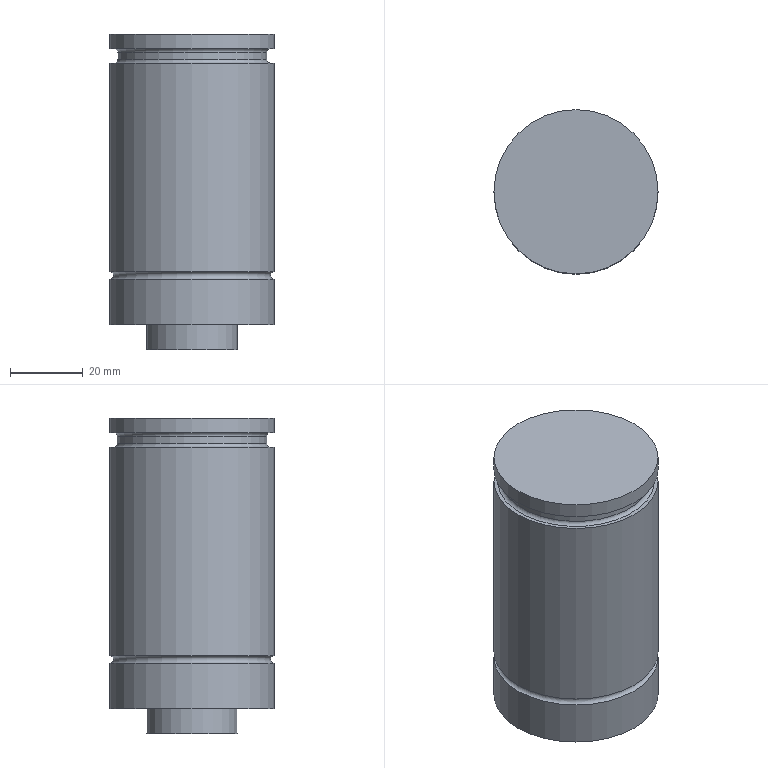Part | NX | features solid 2 | 1 solid | 13 faces | box 45.2 x 45.2 x 87 mm | volume 130556 mm3 | cylinder 5 | plane 5 | torus 3 | commonest cylinder face diameters 45.2 x3 25 x1 41.2 x1
STEP:
#1=CARTESIAN_POINT('',(-1182.6,-595.,9.));
#2=VERTEX_POINT('',#1);
#3=CARTESIAN_POINT('',(-1160.,-595.,9.));
#4=DIRECTION('',(0.,0.,-1.));
#5=DIRECTION('',(-1.,0.,0.));
#6=AXIS2_PLACEMENT_3D('',#3,#4,#5);
#7=CIRCLE('',#6,22.6);
#8=EDGE_CURVE('',#2,#2,#7,.T.);
#9=ORIENTED_EDGE('',*,*,#8,.T.);
#10=EDGE_LOOP('',(#9));
#11=FACE_BOUND('',#10,.T.);
#12=CARTESIAN_POINT('',(-1137.4,-595.,-48.5));
#13=VERTEX_POINT('',#12);
#14=CARTESIAN_POINT('',(-1160.,-595.,-48.5));
#15=DIRECTION('',(0.,0.,1.));
#16=DIRECTION('',(1.,0.,0.));
#17=AXIS2_PLACEMENT_3D('',#14,#15,#16);
#18=CIRCLE('',#17,22.6);
#19=EDGE_CURVE('',#13,#13,#18,.T.);
#20=ORIENTED_EDGE('',*,*,#19,.T.);
#21=EDGE_LOOP('',(#20));
#22=FACE_BOUND('',#21,.T.);
#23=CARTESIAN_POINT('',(-1160.,-595.,-63.));
#24=DIRECTION('',(0.,0.,1.));
#25=DIRECTION('',(1.,0.,0.));
#26=AXIS2_PLACEMENT_3D('',#23,#24,#25);
#27=CYLINDRICAL_SURFACE('',#26,22.6);
#28=ADVANCED_FACE('',(#11,#22),#27,.T.);
#29=CARTESIAN_POINT('',(-1172.5,-595.,-63.));
#30=VERTEX_POINT('',#29);
#31=CARTESIAN_POINT('',(-1160.,-595.,-63.));
#32=DIRECTION('',(0.,0.,-1.));
#33=DIRECTION('',(-1.,0.,0.));
#34=AXIS2_PLACEMENT_3D('',#31,#32,#33);
#35=CIRCLE('',#34,12.5);
#36=EDGE_CURVE('',#30,#30,#35,.T.);
#37=ORIENTED_EDGE('',*,*,#36,.F.);
#38=EDGE_LOOP('',(#37));
#39=FACE_BOUND('',#38,.T.);
#40=CARTESIAN_POINT('',(-1137.4,-595.,-63.));
#41=VERTEX_POINT('',#40);
#42=CARTESIAN_POINT('',(-1160.,-595.,-63.));
#43=DIRECTION('',(0.,0.,1.));
#44=DIRECTION('',(1.,0.,0.));
#45=AXIS2_PLACEMENT_3D('',#42,#43,#44);
#46=CIRCLE('',#45,22.6);
#47=EDGE_CURVE('',#41,#41,#46,.T.);
#48=ORIENTED_EDGE('',*,*,#47,.F.);
#49=EDGE_LOOP('',(#48));
#50=FACE_BOUND('',#49,.T.);
#51=CARTESIAN_POINT('',(-1160.,-595.,-63.));
#52=DIRECTION('',(0.,0.,-1.));
#53=DIRECTION('',(-1.,0.,0.));
#54=AXIS2_PLACEMENT_3D('',#51,#52,#53);
#55=PLANE('',#54);
#56=ADVANCED_FACE('',(#39,#50),#55,.T.);
#57=CARTESIAN_POINT('',(-1137.4,-595.,-50.5));
#58=VERTEX_POINT('',#57);
#59=CARTESIAN_POINT('',(-1160.,-595.,-50.5));
#60=DIRECTION('',(0.,0.,1.));
#61=DIRECTION('',(1.,0.,0.));
#62=AXIS2_PLACEMENT_3D('',#59,#60,#61);
#63=CIRCLE('',#62,22.6);
#64=EDGE_CURVE('',#58,#58,#63,.T.);
#65=ORIENTED_EDGE('',*,*,#64,.F.);
#66=EDGE_LOOP('',(#65));
#67=FACE_BOUND('',#66,.T.);
#68=ORIENTED_EDGE('',*,*,#47,.T.);
#69=EDGE_LOOP('',(#68));
#70=FACE_BOUND('',#69,.T.);
#71=CARTESIAN_POINT('',(-1160.,-595.,-63.));
#72=DIRECTION('',(0.,0.,1.));
#73=DIRECTION('',(1.,0.,0.));
#74=AXIS2_PLACEMENT_3D('',#71,#72,#73);
#75=CYLINDRICAL_SURFACE('',#74,22.6);
#76=ADVANCED_FACE('',(#67,#70),#75,.T.);
#77=CARTESIAN_POINT('',(-1147.5,-595.,-70.));
#78=VERTEX_POINT('',#77);
#79=CARTESIAN_POINT('',(-1160.,-595.,-70.));
#80=DIRECTION('',(0.,0.,1.));
#81=DIRECTION('',(1.,0.,0.));
#82=AXIS2_PLACEMENT_3D('',#79,#80,#81);
#83=CIRCLE('',#82,12.5);
#84=EDGE_CURVE('',#78,#78,#83,.T.);
#85=ORIENTED_EDGE('',*,*,#84,.F.);
#86=EDGE_LOOP('',(#85));
#87=FACE_BOUND('',#86,.T.);
#88=CARTESIAN_POINT('',(-1160.,-595.,-70.));
#89=DIRECTION('',(0.,0.,-1.));
#90=DIRECTION('',(-1.,0.,0.));
#91=AXIS2_PLACEMENT_3D('',#88,#89,#90);
#92=PLANE('',#91);
#93=ADVANCED_FACE('',(#87),#92,.T.);
#94=ORIENTED_EDGE('',*,*,#36,.T.);
#95=EDGE_LOOP('',(#94));
#96=FACE_BOUND('',#95,.T.);
#97=ORIENTED_EDGE('',*,*,#84,.T.);
#98=EDGE_LOOP('',(#97));
#99=FACE_BOUND('',#98,.T.);
#100=CARTESIAN_POINT('',(-1160.,-595.,-70.));
#101=DIRECTION('',(0.,0.,1.));
#102=DIRECTION('',(1.,0.,0.));
#103=AXIS2_PLACEMENT_3D('',#100,#101,#102);
#104=CYLINDRICAL_SURFACE('',#103,12.5);
#105=ADVANCED_FACE('',(#96,#99),#104,.T.);
#106=ORIENTED_EDGE('',*,*,#19,.F.);
#107=EDGE_LOOP('',(#106));
#108=FACE_BOUND('',#107,.T.);
#109=ORIENTED_EDGE('',*,*,#64,.T.);
#110=EDGE_LOOP('',(#109));
#111=FACE_BOUND('',#110,.T.);
#112=CARTESIAN_POINT('',(-1160.,-595.,-49.5));
#113=DIRECTION('',(0.,0.,-1.));
#114=DIRECTION('',(-1.,0.,0.));
#115=AXIS2_PLACEMENT_3D('',#112,#113,#114);
#116=TOROIDAL_SURFACE('',#115,22.6,1.);
#117=ADVANCED_FACE('',(#108,#111),#116,.F.);
#118=CARTESIAN_POINT('',(-1139.4,-595.,10.));
#119=VERTEX_POINT('',#118);
#120=CARTESIAN_POINT('',(-1160.,-595.,10.));
#121=DIRECTION('',(0.,0.,1.));
#122=DIRECTION('',(1.,0.,0.));
#123=AXIS2_PLACEMENT_3D('',#120,#121,#122);
#124=CIRCLE('',#123,20.6);
#125=EDGE_CURVE('',#119,#119,#124,.T.);
#126=ORIENTED_EDGE('',*,*,#125,.T.);
#127=EDGE_LOOP('',(#126));
#128=FACE_BOUND('',#127,.T.);
#129=CARTESIAN_POINT('',(-1139.4,-595.,12.));
#130=VERTEX_POINT('',#129);
#131=CARTESIAN_POINT('',(-1160.,-595.,12.));
#132=DIRECTION('',(0.,0.,1.));
#133=DIRECTION('',(1.,0.,0.));
#134=AXIS2_PLACEMENT_3D('',#131,#132,#133);
#135=CIRCLE('',#134,20.6);
#136=EDGE_CURVE('',#130,#130,#135,.F.);
#137=ORIENTED_EDGE('',*,*,#136,.T.);
#138=EDGE_LOOP('',(#137));
#139=FACE_BOUND('',#138,.T.);
#140=CARTESIAN_POINT('',(-1160.,-595.,13.));
#141=DIRECTION('',(0.,0.,-1.));
#142=DIRECTION('',(-1.,0.,0.));
#143=AXIS2_PLACEMENT_3D('',#140,#141,#142);
#144=CYLINDRICAL_SURFACE('',#143,20.6);
#145=ADVANCED_FACE('',(#128,#139),#144,.T.);
#146=CARTESIAN_POINT('',(-1138.4,-595.,13.));
#147=VERTEX_POINT('',#146);
#148=CARTESIAN_POINT('',(-1160.,-595.,13.));
#149=DIRECTION('',(0.,0.,1.));
#150=DIRECTION('',(1.,0.,0.));
#151=AXIS2_PLACEMENT_3D('',#148,#149,#150);
#152=CIRCLE('',#151,21.6);
#153=EDGE_CURVE('',#147,#147,#152,.T.);
#154=ORIENTED_EDGE('',*,*,#153,.T.);
#155=EDGE_LOOP('',(#154));
#156=FACE_BOUND('',#155,.T.);
#157=CARTESIAN_POINT('',(-1182.6,-595.,13.));
#158=VERTEX_POINT('',#157);
#159=CARTESIAN_POINT('',(-1160.,-595.,13.));
#160=DIRECTION('',(0.,0.,-1.));
#161=DIRECTION('',(-1.,0.,0.));
#162=AXIS2_PLACEMENT_3D('',#159,#160,#161);
#163=CIRCLE('',#162,22.6);
#164=EDGE_CURVE('',#158,#158,#163,.T.);
#165=ORIENTED_EDGE('',*,*,#164,.T.);
#166=EDGE_LOOP('',(#165));
#167=FACE_BOUND('',#166,.T.);
#168=CARTESIAN_POINT('',(-1160.,-595.,13.));
#169=DIRECTION('',(0.,0.,1.));
#170=DIRECTION('',(1.,0.,0.));
#171=AXIS2_PLACEMENT_3D('',#168,#169,#170);
#172=PLANE('',#171);
#173=ADVANCED_FACE('',(#156,#167),#172,.F.);
#174=CARTESIAN_POINT('',(-1138.4,-595.,9.));
#175=VERTEX_POINT('',#174);
#176=CARTESIAN_POINT('',(-1160.,-595.,9.));
#177=DIRECTION('',(0.,0.,1.));
#178=DIRECTION('',(1.,0.,0.));
#179=AXIS2_PLACEMENT_3D('',#176,#177,#178);
#180=CIRCLE('',#179,21.6);
#181=EDGE_CURVE('',#175,#175,#180,.F.);
#182=ORIENTED_EDGE('',*,*,#181,.T.);
#183=EDGE_LOOP('',(#182));
#184=FACE_BOUND('',#183,.T.);
#185=ORIENTED_EDGE('',*,*,#8,.F.);
#186=EDGE_LOOP('',(#185));
#187=FACE_BOUND('',#186,.T.);
#188=CARTESIAN_POINT('',(-1160.,-595.,9.));
#189=DIRECTION('',(0.,0.,1.));
#190=DIRECTION('',(1.,0.,0.));
#191=AXIS2_PLACEMENT_3D('',#188,#189,#190);
#192=PLANE('',#191);
#193=ADVANCED_FACE('',(#184,#187),#192,.T.);
#194=CARTESIAN_POINT('',(-1182.6,-595.,17.));
#195=VERTEX_POINT('',#194);
#196=CARTESIAN_POINT('',(-1160.,-595.,17.));
#197=DIRECTION('',(0.,0.,-1.));
#198=DIRECTION('',(-1.,0.,0.));
#199=AXIS2_PLACEMENT_3D('',#196,#197,#198);
#200=CIRCLE('',#199,22.6);
#201=EDGE_CURVE('',#195,#195,#200,.T.);
#202=ORIENTED_EDGE('',*,*,#201,.F.);
#203=EDGE_LOOP('',(#202));
#204=FACE_BOUND('',#203,.T.);
#205=CARTESIAN_POINT('',(-1160.,-595.,17.));
#206=DIRECTION('',(0.,0.,1.));
#207=DIRECTION('',(1.,0.,0.));
#208=AXIS2_PLACEMENT_3D('',#205,#206,#207);
#209=PLANE('',#208);
#210=ADVANCED_FACE('',(#204),#209,.T.);
#211=ORIENTED_EDGE('',*,*,#164,.F.);
#212=EDGE_LOOP('',(#211));
#213=FACE_BOUND('',#212,.T.);
#214=ORIENTED_EDGE('',*,*,#201,.T.);
#215=EDGE_LOOP('',(#214));
#216=FACE_BOUND('',#215,.T.);
#217=CARTESIAN_POINT('',(-1160.,-595.,-63.));
#218=DIRECTION('',(0.,0.,1.));
#219=DIRECTION('',(1.,0.,0.));
#220=AXIS2_PLACEMENT_3D('',#217,#218,#219);
#221=CYLINDRICAL_SURFACE('',#220,22.6);
#222=ADVANCED_FACE('',(#213,#216),#221,.T.);
#223=ORIENTED_EDGE('',*,*,#125,.F.);
#224=EDGE_LOOP('',(#223));
#225=FACE_BOUND('',#224,.T.);
#226=ORIENTED_EDGE('',*,*,#181,.F.);
#227=EDGE_LOOP('',(#226));
#228=FACE_BOUND('',#227,.T.);
#229=CARTESIAN_POINT('',(-1160.,-595.,10.));
#230=DIRECTION('',(0.,0.,1.));
#231=DIRECTION('',(1.,0.,0.));
#232=AXIS2_PLACEMENT_3D('',#229,#230,#231);
#233=TOROIDAL_SURFACE('',#232,21.6,1.);
#234=ADVANCED_FACE('',(#225,#228),#233,.F.);
#235=ORIENTED_EDGE('',*,*,#153,.F.);
#236=EDGE_LOOP('',(#235));
#237=FACE_BOUND('',#236,.T.);
#238=ORIENTED_EDGE('',*,*,#136,.F.);
#239=EDGE_LOOP('',(#238));
#240=FACE_BOUND('',#239,.T.);
#241=CARTESIAN_POINT('',(-1160.,-595.,12.));
#242=DIRECTION('',(0.,0.,1.));
#243=DIRECTION('',(1.,0.,0.));
#244=AXIS2_PLACEMENT_3D('',#241,#242,#243);
#245=TOROIDAL_SURFACE('',#244,21.6,1.);
#246=ADVANCED_FACE('',(#237,#240),#245,.F.);
#247=CLOSED_SHELL('',(#28,#56,#76,#93,#105,#117,#145,#173,#193,#210,#222,#234,#246));
#248=MANIFOLD_SOLID_BREP('',#247);
#249=(LENGTH_UNIT()NAMED_UNIT(*)SI_UNIT(.MILLI.,.METRE.));
#250=UNCERTAINTY_MEASURE_WITH_UNIT(LENGTH_MEASURE(0.00001),#249,'','');
#251=(NAMED_UNIT(*)PLANE_ANGLE_UNIT()SI_UNIT($,.RADIAN.));
#252=(NAMED_UNIT(*)SI_UNIT($,.STERADIAN.)SOLID_ANGLE_UNIT());
#253=(GEOMETRIC_REPRESENTATION_CONTEXT(3)GLOBAL_UNCERTAINTY_ASSIGNED_CONTEXT((#250))GLOBAL_UNIT_ASSIGNED_CONTEXT((#249,#251,#252))REPRESENTATION_CONTEXT('',''));
#254=ADVANCED_BREP_SHAPE_REPRESENTATION('',(#248),#253);